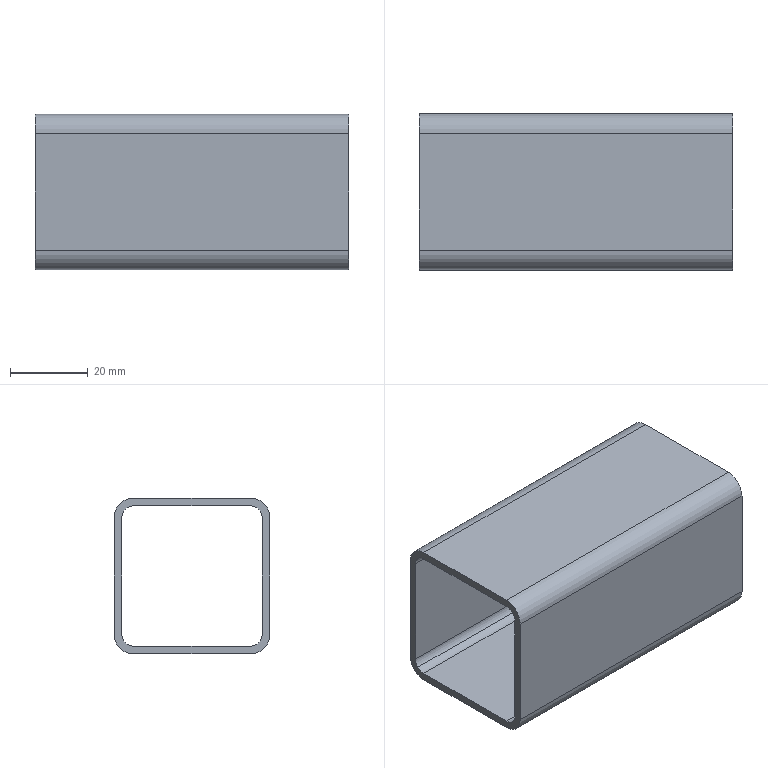Part | NX | features BREP 1 | 1 solid | 22 faces | box 80.5 x 40 x 40 mm | volume 23366 mm3 | cylinder 12 | plane 10 | commonest cylinder face diameters 6 x8 10 x4
STEP:
#1=CARTESIAN_POINT('',(2064.581,-321.621,69.879));
#2=VERTEX_POINT('',#1);
#3=CARTESIAN_POINT('',(2064.581,-319.5,69.));
#4=VERTEX_POINT('',#3);
#5=CARTESIAN_POINT('',(2064.581,-319.5,72.));
#6=DIRECTION('',(1.,0.,0.));
#7=DIRECTION('',(0.,0.,-1.));
#8=AXIS2_PLACEMENT_3D('',#5,#6,#7);
#9=CIRCLE('',#8,3.);
#10=EDGE_CURVE('',#2,#4,#9,.T.);
#11=ORIENTED_EDGE('',*,*,#10,.F.);
#12=CARTESIAN_POINT('',(2064.581,-322.5,72.));
#13=VERTEX_POINT('',#12);
#14=CARTESIAN_POINT('',(2064.581,-319.5,72.));
#15=DIRECTION('',(1.,0.,0.));
#16=DIRECTION('',(0.,0.,-1.));
#17=AXIS2_PLACEMENT_3D('',#14,#15,#16);
#18=CIRCLE('',#17,3.);
#19=EDGE_CURVE('',#13,#2,#18,.T.);
#20=ORIENTED_EDGE('',*,*,#19,.F.);
#21=CARTESIAN_POINT('',(2064.581,-322.5,102.));
#22=VERTEX_POINT('',#21);
#23=CARTESIAN_POINT('',(2064.581,-322.5,87.));
#24=DIRECTION('',(0.,0.,1.));
#25=VECTOR('',#24,1000.);
#26=LINE('',#23,#25);
#27=EDGE_CURVE('',#13,#22,#26,.T.);
#28=ORIENTED_EDGE('',*,*,#27,.T.);
#29=CARTESIAN_POINT('',(2064.581,-321.621,104.121));
#30=VERTEX_POINT('',#29);
#31=CARTESIAN_POINT('',(2064.581,-319.5,102.));
#32=DIRECTION('',(1.,0.,0.));
#33=DIRECTION('',(0.,0.,-1.));
#34=AXIS2_PLACEMENT_3D('',#31,#32,#33);
#35=CIRCLE('',#34,3.);
#36=EDGE_CURVE('',#30,#22,#35,.T.);
#37=ORIENTED_EDGE('',*,*,#36,.F.);
#38=CARTESIAN_POINT('',(2064.581,-319.5,105.));
#39=VERTEX_POINT('',#38);
#40=CARTESIAN_POINT('',(2064.581,-319.5,102.));
#41=DIRECTION('',(1.,0.,0.));
#42=DIRECTION('',(0.,0.,-1.));
#43=AXIS2_PLACEMENT_3D('',#40,#41,#42);
#44=CIRCLE('',#43,3.);
#45=EDGE_CURVE('',#39,#30,#44,.T.);
#46=ORIENTED_EDGE('',*,*,#45,.F.);
#47=CARTESIAN_POINT('',(2064.581,-289.5,105.));
#48=VERTEX_POINT('',#47);
#49=CARTESIAN_POINT('',(2064.581,-304.5,105.));
#50=DIRECTION('',(0.,-1.,0.));
#51=VECTOR('',#50,1000.);
#52=LINE('',#49,#51);
#53=EDGE_CURVE('',#48,#39,#52,.T.);
#54=ORIENTED_EDGE('',*,*,#53,.F.);
#55=CARTESIAN_POINT('',(2064.581,-287.378,104.121));
#56=VERTEX_POINT('',#55);
#57=CARTESIAN_POINT('',(2064.581,-289.5,102.));
#58=DIRECTION('',(1.,0.,0.));
#59=DIRECTION('',(0.,0.,-1.));
#60=AXIS2_PLACEMENT_3D('',#57,#58,#59);
#61=CIRCLE('',#60,3.);
#62=EDGE_CURVE('',#56,#48,#61,.T.);
#63=ORIENTED_EDGE('',*,*,#62,.F.);
#64=CARTESIAN_POINT('',(2064.581,-286.5,102.));
#65=VERTEX_POINT('',#64);
#66=CARTESIAN_POINT('',(2064.581,-289.5,102.));
#67=DIRECTION('',(1.,0.,0.));
#68=DIRECTION('',(0.,0.,-1.));
#69=AXIS2_PLACEMENT_3D('',#66,#67,#68);
#70=CIRCLE('',#69,3.);
#71=EDGE_CURVE('',#65,#56,#70,.T.);
#72=ORIENTED_EDGE('',*,*,#71,.F.);
#73=CARTESIAN_POINT('',(2064.581,-286.5,72.));
#74=VERTEX_POINT('',#73);
#75=CARTESIAN_POINT('',(2064.581,-286.5,87.));
#76=DIRECTION('',(0.,0.,-1.));
#77=VECTOR('',#76,1000.);
#78=LINE('',#75,#77);
#79=EDGE_CURVE('',#65,#74,#78,.T.);
#80=ORIENTED_EDGE('',*,*,#79,.T.);
#81=CARTESIAN_POINT('',(2064.581,-287.378,69.879));
#82=VERTEX_POINT('',#81);
#83=CARTESIAN_POINT('',(2064.581,-289.5,72.));
#84=DIRECTION('',(1.,0.,0.));
#85=DIRECTION('',(0.,0.,-1.));
#86=AXIS2_PLACEMENT_3D('',#83,#84,#85);
#87=CIRCLE('',#86,3.);
#88=EDGE_CURVE('',#82,#74,#87,.T.);
#89=ORIENTED_EDGE('',*,*,#88,.F.);
#90=CARTESIAN_POINT('',(2064.581,-289.5,69.));
#91=VERTEX_POINT('',#90);
#92=CARTESIAN_POINT('',(2064.581,-289.5,72.));
#93=DIRECTION('',(1.,0.,0.));
#94=DIRECTION('',(0.,0.,-1.));
#95=AXIS2_PLACEMENT_3D('',#92,#93,#94);
#96=CIRCLE('',#95,3.);
#97=EDGE_CURVE('',#91,#82,#96,.T.);
#98=ORIENTED_EDGE('',*,*,#97,.F.);
#99=CARTESIAN_POINT('',(2064.581,-304.5,69.));
#100=DIRECTION('',(0.,1.,0.));
#101=VECTOR('',#100,1000.);
#102=LINE('',#99,#101);
#103=EDGE_CURVE('',#4,#91,#102,.T.);
#104=ORIENTED_EDGE('',*,*,#103,.F.);
#105=EDGE_LOOP('',(#11,#20,#28,#37,#46,#54,#63,#72,#80,#89,#98,#104));
#106=FACE_BOUND('',#105,.T.);
#107=CARTESIAN_POINT('',(2064.581,-319.5,67.));
#108=VERTEX_POINT('',#107);
#109=CARTESIAN_POINT('',(2064.581,-289.5,67.));
#110=VERTEX_POINT('',#109);
#111=CARTESIAN_POINT('',(2064.581,-304.5,67.));
#112=DIRECTION('',(0.,1.,0.));
#113=VECTOR('',#112,1000.);
#114=LINE('',#111,#113);
#115=EDGE_CURVE('',#108,#110,#114,.T.);
#116=ORIENTED_EDGE('',*,*,#115,.T.);
#117=CARTESIAN_POINT('',(2064.581,-284.5,72.));
#118=VERTEX_POINT('',#117);
#119=CARTESIAN_POINT('',(2064.581,-289.5,72.));
#120=DIRECTION('',(1.,0.,0.));
#121=DIRECTION('',(0.,0.,-1.));
#122=AXIS2_PLACEMENT_3D('',#119,#120,#121);
#123=CIRCLE('',#122,5.);
#124=EDGE_CURVE('',#110,#118,#123,.T.);
#125=ORIENTED_EDGE('',*,*,#124,.T.);
#126=CARTESIAN_POINT('',(2064.581,-284.5,102.));
#127=VERTEX_POINT('',#126);
#128=CARTESIAN_POINT('',(2064.581,-284.5,87.));
#129=DIRECTION('',(0.,0.,-1.));
#130=VECTOR('',#129,1000.);
#131=LINE('',#128,#130);
#132=EDGE_CURVE('',#127,#118,#131,.T.);
#133=ORIENTED_EDGE('',*,*,#132,.F.);
#134=CARTESIAN_POINT('',(2064.581,-289.5,107.));
#135=VERTEX_POINT('',#134);
#136=CARTESIAN_POINT('',(2064.581,-289.5,102.));
#137=DIRECTION('',(1.,0.,0.));
#138=DIRECTION('',(0.,0.,-1.));
#139=AXIS2_PLACEMENT_3D('',#136,#137,#138);
#140=CIRCLE('',#139,5.);
#141=EDGE_CURVE('',#127,#135,#140,.T.);
#142=ORIENTED_EDGE('',*,*,#141,.T.);
#143=CARTESIAN_POINT('',(2064.581,-319.5,107.));
#144=VERTEX_POINT('',#143);
#145=CARTESIAN_POINT('',(2064.581,-304.5,107.));
#146=DIRECTION('',(0.,-1.,0.));
#147=VECTOR('',#146,1000.);
#148=LINE('',#145,#147);
#149=EDGE_CURVE('',#135,#144,#148,.T.);
#150=ORIENTED_EDGE('',*,*,#149,.T.);
#151=CARTESIAN_POINT('',(2064.581,-324.5,102.));
#152=VERTEX_POINT('',#151);
#153=CARTESIAN_POINT('',(2064.581,-319.5,102.));
#154=DIRECTION('',(1.,0.,0.));
#155=DIRECTION('',(0.,0.,-1.));
#156=AXIS2_PLACEMENT_3D('',#153,#154,#155);
#157=CIRCLE('',#156,5.);
#158=EDGE_CURVE('',#144,#152,#157,.T.);
#159=ORIENTED_EDGE('',*,*,#158,.T.);
#160=CARTESIAN_POINT('',(2064.581,-324.5,72.));
#161=VERTEX_POINT('',#160);
#162=CARTESIAN_POINT('',(2064.581,-324.5,87.));
#163=DIRECTION('',(0.,0.,1.));
#164=VECTOR('',#163,1000.);
#165=LINE('',#162,#164);
#166=EDGE_CURVE('',#161,#152,#165,.T.);
#167=ORIENTED_EDGE('',*,*,#166,.F.);
#168=CARTESIAN_POINT('',(2064.581,-319.5,72.));
#169=DIRECTION('',(1.,0.,0.));
#170=DIRECTION('',(0.,0.,-1.));
#171=AXIS2_PLACEMENT_3D('',#168,#169,#170);
#172=CIRCLE('',#171,5.);
#173=EDGE_CURVE('',#161,#108,#172,.T.);
#174=ORIENTED_EDGE('',*,*,#173,.T.);
#175=EDGE_LOOP('',(#116,#125,#133,#142,#150,#159,#167,#174));
#176=FACE_BOUND('',#175,.T.);
#177=CARTESIAN_POINT('',(2064.581,-306.25,87.));
#178=DIRECTION('',(1.,0.,0.));
#179=DIRECTION('',(0.,0.,-1.));
#180=AXIS2_PLACEMENT_3D('',#177,#178,#179);
#181=PLANE('',#180);
#182=ADVANCED_FACE('',(#106,#176),#181,.T.);
#183=CARTESIAN_POINT('',(1984.081,-286.5,72.));
#184=VERTEX_POINT('',#183);
#185=CARTESIAN_POINT('',(993.946,-286.5,72.));
#186=DIRECTION('',(1.,0.,0.));
#187=VECTOR('',#186,1000.);
#188=LINE('',#185,#187);
#189=EDGE_CURVE('',#184,#74,#188,.T.);
#190=ORIENTED_EDGE('',*,*,#189,.T.);
#191=ORIENTED_EDGE('',*,*,#79,.F.);
#192=CARTESIAN_POINT('',(1984.081,-286.5,102.));
#193=VERTEX_POINT('',#192);
#194=CARTESIAN_POINT('',(993.946,-286.5,102.));
#195=DIRECTION('',(1.,0.,0.));
#196=VECTOR('',#195,1000.);
#197=LINE('',#194,#196);
#198=EDGE_CURVE('',#193,#65,#197,.T.);
#199=ORIENTED_EDGE('',*,*,#198,.F.);
#200=CARTESIAN_POINT('',(1984.081,-286.5,87.));
#201=DIRECTION('',(0.,0.,-1.));
#202=VECTOR('',#201,1000.);
#203=LINE('',#200,#202);
#204=EDGE_CURVE('',#193,#184,#203,.T.);
#205=ORIENTED_EDGE('',*,*,#204,.T.);
#206=EDGE_LOOP('',(#190,#191,#199,#205));
#207=FACE_BOUND('',#206,.T.);
#208=CARTESIAN_POINT('',(601.965,-286.5,127.));
#209=DIRECTION('',(0.,-1.,0.));
#210=DIRECTION('',(0.,0.,-1.));
#211=AXIS2_PLACEMENT_3D('',#208,#209,#210);
#212=PLANE('',#211);
#213=ADVANCED_FACE('',(#207),#212,.T.);
#214=ORIENTED_EDGE('',*,*,#88,.T.);
#215=ORIENTED_EDGE('',*,*,#189,.F.);
#216=CARTESIAN_POINT('',(1984.081,-287.378,69.879));
#217=VERTEX_POINT('',#216);
#218=CARTESIAN_POINT('',(1984.081,-289.5,72.));
#219=DIRECTION('',(1.,0.,0.));
#220=DIRECTION('',(0.,0.,-1.));
#221=AXIS2_PLACEMENT_3D('',#218,#219,#220);
#222=CIRCLE('',#221,3.);
#223=EDGE_CURVE('',#217,#184,#222,.T.);
#224=ORIENTED_EDGE('',*,*,#223,.F.);
#225=CARTESIAN_POINT('',(993.946,-287.378,69.879));
#226=DIRECTION('',(1.,0.,0.));
#227=VECTOR('',#226,1000.);
#228=LINE('',#225,#227);
#229=EDGE_CURVE('',#217,#82,#228,.T.);
#230=ORIENTED_EDGE('',*,*,#229,.T.);
#231=EDGE_LOOP('',(#214,#215,#224,#230));
#232=FACE_BOUND('',#231,.T.);
#233=CARTESIAN_POINT('',(993.946,-289.5,72.));
#234=DIRECTION('',(1.,0.,0.));
#235=DIRECTION('',(0.,0.7071,-0.7071));
#236=AXIS2_PLACEMENT_3D('',#233,#234,#235);
#237=CYLINDRICAL_SURFACE('',#236,3.);
#238=ADVANCED_FACE('',(#232),#237,.F.);
#239=CARTESIAN_POINT('',(1984.081,-289.5,69.));
#240=VERTEX_POINT('',#239);
#241=CARTESIAN_POINT('',(1984.081,-289.5,72.));
#242=DIRECTION('',(1.,0.,0.));
#243=DIRECTION('',(0.,0.,-1.));
#244=AXIS2_PLACEMENT_3D('',#241,#242,#243);
#245=CIRCLE('',#244,3.);
#246=EDGE_CURVE('',#240,#217,#245,.T.);
#247=ORIENTED_EDGE('',*,*,#246,.F.);
#248=CARTESIAN_POINT('',(2024.331,-289.5,69.));
#249=DIRECTION('',(1.,0.,0.));
#250=VECTOR('',#249,1000.);
#251=LINE('',#248,#250);
#252=EDGE_CURVE('',#240,#91,#251,.T.);
#253=ORIENTED_EDGE('',*,*,#252,.T.);
#254=ORIENTED_EDGE('',*,*,#97,.T.);
#255=ORIENTED_EDGE('',*,*,#229,.F.);
#256=EDGE_LOOP('',(#247,#253,#254,#255));
#257=FACE_BOUND('',#256,.T.);
#258=CARTESIAN_POINT('',(993.946,-289.5,72.));
#259=DIRECTION('',(1.,0.,0.));
#260=DIRECTION('',(0.,-0.7071,0.7071));
#261=AXIS2_PLACEMENT_3D('',#258,#259,#260);
#262=CYLINDRICAL_SURFACE('',#261,3.);
#263=ADVANCED_FACE('',(#257),#262,.F.);
#264=CARTESIAN_POINT('',(1984.081,-319.5,69.));
#265=VERTEX_POINT('',#264);
#266=CARTESIAN_POINT('',(1984.081,-304.5,69.));
#267=DIRECTION('',(0.,1.,0.));
#268=VECTOR('',#267,1000.);
#269=LINE('',#266,#268);
#270=EDGE_CURVE('',#265,#240,#269,.T.);
#271=ORIENTED_EDGE('',*,*,#270,.F.);
#272=CARTESIAN_POINT('',(993.946,-319.5,69.));
#273=DIRECTION('',(1.,0.,0.));
#274=VECTOR('',#273,1000.);
#275=LINE('',#272,#274);
#276=EDGE_CURVE('',#265,#4,#275,.T.);
#277=ORIENTED_EDGE('',*,*,#276,.T.);
#278=ORIENTED_EDGE('',*,*,#103,.T.);
#279=ORIENTED_EDGE('',*,*,#252,.F.);
#280=EDGE_LOOP('',(#271,#277,#278,#279));
#281=FACE_BOUND('',#280,.T.);
#282=CARTESIAN_POINT('',(601.965,-344.5,69.));
#283=DIRECTION('',(0.,0.,-1.));
#284=DIRECTION('',(0.,1.,0.));
#285=AXIS2_PLACEMENT_3D('',#282,#283,#284);
#286=PLANE('',#285);
#287=ADVANCED_FACE('',(#281),#286,.F.);
#288=ORIENTED_EDGE('',*,*,#10,.T.);
#289=ORIENTED_EDGE('',*,*,#276,.F.);
#290=CARTESIAN_POINT('',(1984.081,-321.621,69.879));
#291=VERTEX_POINT('',#290);
#292=CARTESIAN_POINT('',(1984.081,-319.5,72.));
#293=DIRECTION('',(1.,0.,0.));
#294=DIRECTION('',(0.,0.,-1.));
#295=AXIS2_PLACEMENT_3D('',#292,#293,#294);
#296=CIRCLE('',#295,3.);
#297=EDGE_CURVE('',#291,#265,#296,.T.);
#298=ORIENTED_EDGE('',*,*,#297,.F.);
#299=CARTESIAN_POINT('',(993.946,-321.621,69.879));
#300=DIRECTION('',(1.,0.,0.));
#301=VECTOR('',#300,1000.);
#302=LINE('',#299,#301);
#303=EDGE_CURVE('',#291,#2,#302,.T.);
#304=ORIENTED_EDGE('',*,*,#303,.T.);
#305=EDGE_LOOP('',(#288,#289,#298,#304));
#306=FACE_BOUND('',#305,.T.);
#307=CARTESIAN_POINT('',(993.946,-319.5,72.));
#308=DIRECTION('',(1.,0.,0.));
#309=DIRECTION('',(0.,-0.7071,-0.7071));
#310=AXIS2_PLACEMENT_3D('',#307,#308,#309);
#311=CYLINDRICAL_SURFACE('',#310,3.);
#312=ADVANCED_FACE('',(#306),#311,.F.);
#313=CARTESIAN_POINT('',(1984.081,-322.5,72.));
#314=VERTEX_POINT('',#313);
#315=CARTESIAN_POINT('',(1984.081,-319.5,72.));
#316=DIRECTION('',(1.,0.,0.));
#317=DIRECTION('',(0.,0.,-1.));
#318=AXIS2_PLACEMENT_3D('',#315,#316,#317);
#319=CIRCLE('',#318,3.);
#320=EDGE_CURVE('',#314,#291,#319,.T.);
#321=ORIENTED_EDGE('',*,*,#320,.F.);
#322=CARTESIAN_POINT('',(2024.331,-322.5,72.));
#323=DIRECTION('',(1.,0.,0.));
#324=VECTOR('',#323,1000.);
#325=LINE('',#322,#324);
#326=EDGE_CURVE('',#314,#13,#325,.T.);
#327=ORIENTED_EDGE('',*,*,#326,.T.);
#328=ORIENTED_EDGE('',*,*,#19,.T.);
#329=ORIENTED_EDGE('',*,*,#303,.F.);
#330=EDGE_LOOP('',(#321,#327,#328,#329));
#331=FACE_BOUND('',#330,.T.);
#332=CARTESIAN_POINT('',(993.946,-319.5,72.));
#333=DIRECTION('',(1.,0.,0.));
#334=DIRECTION('',(0.,0.7071,0.7071));
#335=AXIS2_PLACEMENT_3D('',#332,#333,#334);
#336=CYLINDRICAL_SURFACE('',#335,3.);
#337=ADVANCED_FACE('',(#331),#336,.F.);
#338=CARTESIAN_POINT('',(1984.081,-322.5,102.));
#339=VERTEX_POINT('',#338);
#340=CARTESIAN_POINT('',(993.946,-322.5,102.));
#341=DIRECTION('',(1.,0.,0.));
#342=VECTOR('',#341,1000.);
#343=LINE('',#340,#342);
#344=EDGE_CURVE('',#339,#22,#343,.T.);
#345=ORIENTED_EDGE('',*,*,#344,.T.);
#346=ORIENTED_EDGE('',*,*,#27,.F.);
#347=ORIENTED_EDGE('',*,*,#326,.F.);
#348=CARTESIAN_POINT('',(1984.081,-322.5,87.));
#349=DIRECTION('',(0.,0.,1.));
#350=VECTOR('',#349,1000.);
#351=LINE('',#348,#350);
#352=EDGE_CURVE('',#314,#339,#351,.T.);
#353=ORIENTED_EDGE('',*,*,#352,.T.);
#354=EDGE_LOOP('',(#345,#346,#347,#353));
#355=FACE_BOUND('',#354,.T.);
#356=CARTESIAN_POINT('',(601.965,-322.5,47.));
#357=DIRECTION('',(0.,1.,0.));
#358=DIRECTION('',(0.,0.,1.));
#359=AXIS2_PLACEMENT_3D('',#356,#357,#358);
#360=PLANE('',#359);
#361=ADVANCED_FACE('',(#355),#360,.T.);
#362=ORIENTED_EDGE('',*,*,#36,.T.);
#363=ORIENTED_EDGE('',*,*,#344,.F.);
#364=CARTESIAN_POINT('',(1984.081,-321.621,104.121));
#365=VERTEX_POINT('',#364);
#366=CARTESIAN_POINT('',(1984.081,-319.5,102.));
#367=DIRECTION('',(1.,0.,0.));
#368=DIRECTION('',(0.,0.,-1.));
#369=AXIS2_PLACEMENT_3D('',#366,#367,#368);
#370=CIRCLE('',#369,3.);
#371=EDGE_CURVE('',#365,#339,#370,.T.);
#372=ORIENTED_EDGE('',*,*,#371,.F.);
#373=CARTESIAN_POINT('',(993.946,-321.621,104.121));
#374=DIRECTION('',(1.,0.,0.));
#375=VECTOR('',#374,1000.);
#376=LINE('',#373,#375);
#377=EDGE_CURVE('',#365,#30,#376,.T.);
#378=ORIENTED_EDGE('',*,*,#377,.T.);
#379=EDGE_LOOP('',(#362,#363,#372,#378));
#380=FACE_BOUND('',#379,.T.);
#381=CARTESIAN_POINT('',(993.946,-319.5,102.));
#382=DIRECTION('',(1.,0.,0.));
#383=DIRECTION('',(0.,-0.7071,0.7071));
#384=AXIS2_PLACEMENT_3D('',#381,#382,#383);
#385=CYLINDRICAL_SURFACE('',#384,3.);
#386=ADVANCED_FACE('',(#380),#385,.F.);
#387=CARTESIAN_POINT('',(1984.081,-319.5,105.));
#388=VERTEX_POINT('',#387);
#389=CARTESIAN_POINT('',(1984.081,-319.5,102.));
#390=DIRECTION('',(1.,0.,0.));
#391=DIRECTION('',(0.,0.,-1.));
#392=AXIS2_PLACEMENT_3D('',#389,#390,#391);
#393=CIRCLE('',#392,3.);
#394=EDGE_CURVE('',#388,#365,#393,.T.);
#395=ORIENTED_EDGE('',*,*,#394,.F.);
#396=CARTESIAN_POINT('',(2024.331,-319.5,105.));
#397=DIRECTION('',(1.,0.,0.));
#398=VECTOR('',#397,1000.);
#399=LINE('',#396,#398);
#400=EDGE_CURVE('',#388,#39,#399,.T.);
#401=ORIENTED_EDGE('',*,*,#400,.T.);
#402=ORIENTED_EDGE('',*,*,#45,.T.);
#403=ORIENTED_EDGE('',*,*,#377,.F.);
#404=EDGE_LOOP('',(#395,#401,#402,#403));
#405=FACE_BOUND('',#404,.T.);
#406=CARTESIAN_POINT('',(993.946,-319.5,102.));
#407=DIRECTION('',(1.,0.,0.));
#408=DIRECTION('',(0.,0.7071,-0.7071));
#409=AXIS2_PLACEMENT_3D('',#406,#407,#408);
#410=CYLINDRICAL_SURFACE('',#409,3.);
#411=ADVANCED_FACE('',(#405),#410,.F.);
#412=CARTESIAN_POINT('',(1984.081,-289.5,105.));
#413=VERTEX_POINT('',#412);
#414=CARTESIAN_POINT('',(1984.081,-304.5,105.));
#415=DIRECTION('',(0.,-1.,0.));
#416=VECTOR('',#415,1000.);
#417=LINE('',#414,#416);
#418=EDGE_CURVE('',#413,#388,#417,.T.);
#419=ORIENTED_EDGE('',*,*,#418,.F.);
#420=CARTESIAN_POINT('',(993.946,-289.5,105.));
#421=DIRECTION('',(1.,0.,0.));
#422=VECTOR('',#421,1000.);
#423=LINE('',#420,#422);
#424=EDGE_CURVE('',#413,#48,#423,.T.);
#425=ORIENTED_EDGE('',*,*,#424,.T.);
#426=ORIENTED_EDGE('',*,*,#53,.T.);
#427=ORIENTED_EDGE('',*,*,#400,.F.);
#428=EDGE_LOOP('',(#419,#425,#426,#427));
#429=FACE_BOUND('',#428,.T.);
#430=CARTESIAN_POINT('',(601.965,-264.5,105.));
#431=DIRECTION('',(0.,0.,1.));
#432=DIRECTION('',(0.,-1.,0.));
#433=AXIS2_PLACEMENT_3D('',#430,#431,#432);
#434=PLANE('',#433);
#435=ADVANCED_FACE('',(#429),#434,.F.);
#436=ORIENTED_EDGE('',*,*,#62,.T.);
#437=ORIENTED_EDGE('',*,*,#424,.F.);
#438=CARTESIAN_POINT('',(1984.081,-287.378,104.121));
#439=VERTEX_POINT('',#438);
#440=CARTESIAN_POINT('',(1984.081,-289.5,102.));
#441=DIRECTION('',(1.,0.,0.));
#442=DIRECTION('',(0.,0.,-1.));
#443=AXIS2_PLACEMENT_3D('',#440,#441,#442);
#444=CIRCLE('',#443,3.);
#445=EDGE_CURVE('',#439,#413,#444,.T.);
#446=ORIENTED_EDGE('',*,*,#445,.F.);
#447=CARTESIAN_POINT('',(993.946,-287.378,104.121));
#448=DIRECTION('',(1.,0.,0.));
#449=VECTOR('',#448,1000.);
#450=LINE('',#447,#449);
#451=EDGE_CURVE('',#439,#56,#450,.T.);
#452=ORIENTED_EDGE('',*,*,#451,.T.);
#453=EDGE_LOOP('',(#436,#437,#446,#452));
#454=FACE_BOUND('',#453,.T.);
#455=CARTESIAN_POINT('',(993.946,-289.5,102.));
#456=DIRECTION('',(1.,0.,0.));
#457=DIRECTION('',(0.,0.7071,0.7071));
#458=AXIS2_PLACEMENT_3D('',#455,#456,#457);
#459=CYLINDRICAL_SURFACE('',#458,3.);
#460=ADVANCED_FACE('',(#454),#459,.F.);
#461=CARTESIAN_POINT('',(1984.081,-289.5,102.));
#462=DIRECTION('',(1.,0.,0.));
#463=DIRECTION('',(0.,0.,-1.));
#464=AXIS2_PLACEMENT_3D('',#461,#462,#463);
#465=CIRCLE('',#464,3.);
#466=EDGE_CURVE('',#193,#439,#465,.T.);
#467=ORIENTED_EDGE('',*,*,#466,.F.);
#468=ORIENTED_EDGE('',*,*,#198,.T.);
#469=ORIENTED_EDGE('',*,*,#71,.T.);
#470=ORIENTED_EDGE('',*,*,#451,.F.);
#471=EDGE_LOOP('',(#467,#468,#469,#470));
#472=FACE_BOUND('',#471,.T.);
#473=CARTESIAN_POINT('',(993.946,-289.5,102.));
#474=DIRECTION('',(1.,0.,0.));
#475=DIRECTION('',(0.,-0.7071,-0.7071));
#476=AXIS2_PLACEMENT_3D('',#473,#474,#475);
#477=CYLINDRICAL_SURFACE('',#476,3.);
#478=ADVANCED_FACE('',(#472),#477,.F.);
#479=CARTESIAN_POINT('',(1984.081,-289.5,107.));
#480=VERTEX_POINT('',#479);
#481=CARTESIAN_POINT('',(2024.331,-289.5,107.));
#482=DIRECTION('',(1.,0.,0.));
#483=VECTOR('',#482,1000.);
#484=LINE('',#481,#483);
#485=EDGE_CURVE('',#480,#135,#484,.T.);
#486=ORIENTED_EDGE('',*,*,#485,.T.);
#487=ORIENTED_EDGE('',*,*,#141,.F.);
#488=CARTESIAN_POINT('',(1984.081,-284.5,102.));
#489=VERTEX_POINT('',#488);
#490=CARTESIAN_POINT('',(2024.331,-284.5,102.));
#491=DIRECTION('',(1.,0.,0.));
#492=VECTOR('',#491,1000.);
#493=LINE('',#490,#492);
#494=EDGE_CURVE('',#489,#127,#493,.T.);
#495=ORIENTED_EDGE('',*,*,#494,.F.);
#496=CARTESIAN_POINT('',(1984.081,-289.5,102.));
#497=DIRECTION('',(1.,0.,0.));
#498=DIRECTION('',(0.,0.,-1.));
#499=AXIS2_PLACEMENT_3D('',#496,#497,#498);
#500=CIRCLE('',#499,5.);
#501=EDGE_CURVE('',#489,#480,#500,.T.);
#502=ORIENTED_EDGE('',*,*,#501,.T.);
#503=EDGE_LOOP('',(#486,#487,#495,#502));
#504=FACE_BOUND('',#503,.T.);
#505=CARTESIAN_POINT('',(993.946,-289.5,102.));
#506=DIRECTION('',(1.,0.,0.));
#507=DIRECTION('',(0.,1.,0.));
#508=AXIS2_PLACEMENT_3D('',#505,#506,#507);
#509=CYLINDRICAL_SURFACE('',#508,5.);
#510=ADVANCED_FACE('',(#504),#509,.T.);
#511=CARTESIAN_POINT('',(1984.081,-319.5,107.));
#512=VERTEX_POINT('',#511);
#513=CARTESIAN_POINT('',(993.946,-319.5,107.));
#514=DIRECTION('',(1.,0.,0.));
#515=VECTOR('',#514,1000.);
#516=LINE('',#513,#515);
#517=EDGE_CURVE('',#512,#144,#516,.T.);
#518=ORIENTED_EDGE('',*,*,#517,.T.);
#519=ORIENTED_EDGE('',*,*,#149,.F.);
#520=ORIENTED_EDGE('',*,*,#485,.F.);
#521=CARTESIAN_POINT('',(1984.081,-304.5,107.));
#522=DIRECTION('',(0.,-1.,0.));
#523=VECTOR('',#522,1000.);
#524=LINE('',#521,#523);
#525=EDGE_CURVE('',#480,#512,#524,.T.);
#526=ORIENTED_EDGE('',*,*,#525,.T.);
#527=EDGE_LOOP('',(#518,#519,#520,#526));
#528=FACE_BOUND('',#527,.T.);
#529=CARTESIAN_POINT('',(601.965,-264.5,107.));
#530=DIRECTION('',(0.,0.,1.));
#531=DIRECTION('',(0.,-1.,0.));
#532=AXIS2_PLACEMENT_3D('',#529,#530,#531);
#533=PLANE('',#532);
#534=ADVANCED_FACE('',(#528),#533,.T.);
#535=CARTESIAN_POINT('',(1984.081,-324.5,102.));
#536=VERTEX_POINT('',#535);
#537=CARTESIAN_POINT('',(2024.331,-324.5,102.));
#538=DIRECTION('',(1.,0.,0.));
#539=VECTOR('',#538,1000.);
#540=LINE('',#537,#539);
#541=EDGE_CURVE('',#536,#152,#540,.T.);
#542=ORIENTED_EDGE('',*,*,#541,.T.);
#543=ORIENTED_EDGE('',*,*,#158,.F.);
#544=ORIENTED_EDGE('',*,*,#517,.F.);
#545=CARTESIAN_POINT('',(1984.081,-319.5,102.));
#546=DIRECTION('',(1.,0.,0.));
#547=DIRECTION('',(0.,0.,-1.));
#548=AXIS2_PLACEMENT_3D('',#545,#546,#547);
#549=CIRCLE('',#548,5.);
#550=EDGE_CURVE('',#512,#536,#549,.T.);
#551=ORIENTED_EDGE('',*,*,#550,.T.);
#552=EDGE_LOOP('',(#542,#543,#544,#551));
#553=FACE_BOUND('',#552,.T.);
#554=CARTESIAN_POINT('',(993.946,-319.5,102.));
#555=DIRECTION('',(1.,0.,0.));
#556=DIRECTION('',(0.,0.,1.));
#557=AXIS2_PLACEMENT_3D('',#554,#555,#556);
#558=CYLINDRICAL_SURFACE('',#557,5.);
#559=ADVANCED_FACE('',(#553),#558,.T.);
#560=CARTESIAN_POINT('',(1984.081,-324.5,72.));
#561=VERTEX_POINT('',#560);
#562=CARTESIAN_POINT('',(1984.081,-324.5,87.));
#563=DIRECTION('',(0.,0.,1.));
#564=VECTOR('',#563,1000.);
#565=LINE('',#562,#564);
#566=EDGE_CURVE('',#561,#536,#565,.T.);
#567=ORIENTED_EDGE('',*,*,#566,.F.);
#568=CARTESIAN_POINT('',(993.946,-324.5,72.));
#569=DIRECTION('',(1.,0.,0.));
#570=VECTOR('',#569,1000.);
#571=LINE('',#568,#570);
#572=EDGE_CURVE('',#561,#161,#571,.T.);
#573=ORIENTED_EDGE('',*,*,#572,.T.);
#574=ORIENTED_EDGE('',*,*,#166,.T.);
#575=ORIENTED_EDGE('',*,*,#541,.F.);
#576=EDGE_LOOP('',(#567,#573,#574,#575));
#577=FACE_BOUND('',#576,.T.);
#578=CARTESIAN_POINT('',(601.965,-324.5,47.));
#579=DIRECTION('',(0.,1.,0.));
#580=DIRECTION('',(0.,0.,1.));
#581=AXIS2_PLACEMENT_3D('',#578,#579,#580);
#582=PLANE('',#581);
#583=ADVANCED_FACE('',(#577),#582,.F.);
#584=CARTESIAN_POINT('',(1984.081,-319.5,67.));
#585=VERTEX_POINT('',#584);
#586=CARTESIAN_POINT('',(2024.331,-319.5,67.));
#587=DIRECTION('',(1.,0.,0.));
#588=VECTOR('',#587,1000.);
#589=LINE('',#586,#588);
#590=EDGE_CURVE('',#585,#108,#589,.T.);
#591=ORIENTED_EDGE('',*,*,#590,.T.);
#592=ORIENTED_EDGE('',*,*,#173,.F.);
#593=ORIENTED_EDGE('',*,*,#572,.F.);
#594=CARTESIAN_POINT('',(1984.081,-319.5,72.));
#595=DIRECTION('',(1.,0.,0.));
#596=DIRECTION('',(0.,0.,-1.));
#597=AXIS2_PLACEMENT_3D('',#594,#595,#596);
#598=CIRCLE('',#597,5.);
#599=EDGE_CURVE('',#561,#585,#598,.T.);
#600=ORIENTED_EDGE('',*,*,#599,.T.);
#601=EDGE_LOOP('',(#591,#592,#593,#600));
#602=FACE_BOUND('',#601,.T.);
#603=CARTESIAN_POINT('',(993.946,-319.5,72.));
#604=DIRECTION('',(1.,0.,0.));
#605=DIRECTION('',(0.,-1.,0.));
#606=AXIS2_PLACEMENT_3D('',#603,#604,#605);
#607=CYLINDRICAL_SURFACE('',#606,5.);
#608=ADVANCED_FACE('',(#602),#607,.T.);
#609=CARTESIAN_POINT('',(1984.081,-289.5,67.));
#610=VERTEX_POINT('',#609);
#611=CARTESIAN_POINT('',(993.946,-289.5,67.));
#612=DIRECTION('',(1.,0.,0.));
#613=VECTOR('',#612,1000.);
#614=LINE('',#611,#613);
#615=EDGE_CURVE('',#610,#110,#614,.T.);
#616=ORIENTED_EDGE('',*,*,#615,.T.);
#617=ORIENTED_EDGE('',*,*,#115,.F.);
#618=ORIENTED_EDGE('',*,*,#590,.F.);
#619=CARTESIAN_POINT('',(1984.081,-304.5,67.));
#620=DIRECTION('',(0.,1.,0.));
#621=VECTOR('',#620,1000.);
#622=LINE('',#619,#621);
#623=EDGE_CURVE('',#585,#610,#622,.T.);
#624=ORIENTED_EDGE('',*,*,#623,.T.);
#625=EDGE_LOOP('',(#616,#617,#618,#624));
#626=FACE_BOUND('',#625,.T.);
#627=CARTESIAN_POINT('',(601.965,-344.5,67.));
#628=DIRECTION('',(0.,0.,-1.));
#629=DIRECTION('',(0.,1.,0.));
#630=AXIS2_PLACEMENT_3D('',#627,#628,#629);
#631=PLANE('',#630);
#632=ADVANCED_FACE('',(#626),#631,.T.);
#633=CARTESIAN_POINT('',(1984.081,-284.5,72.));
#634=VERTEX_POINT('',#633);
#635=CARTESIAN_POINT('',(2024.331,-284.5,72.));
#636=DIRECTION('',(1.,0.,0.));
#637=VECTOR('',#636,1000.);
#638=LINE('',#635,#637);
#639=EDGE_CURVE('',#634,#118,#638,.T.);
#640=ORIENTED_EDGE('',*,*,#639,.T.);
#641=ORIENTED_EDGE('',*,*,#124,.F.);
#642=ORIENTED_EDGE('',*,*,#615,.F.);
#643=CARTESIAN_POINT('',(1984.081,-289.5,72.));
#644=DIRECTION('',(1.,0.,0.));
#645=DIRECTION('',(0.,0.,-1.));
#646=AXIS2_PLACEMENT_3D('',#643,#644,#645);
#647=CIRCLE('',#646,5.);
#648=EDGE_CURVE('',#610,#634,#647,.T.);
#649=ORIENTED_EDGE('',*,*,#648,.T.);
#650=EDGE_LOOP('',(#640,#641,#642,#649));
#651=FACE_BOUND('',#650,.T.);
#652=CARTESIAN_POINT('',(993.946,-289.5,72.));
#653=DIRECTION('',(1.,0.,0.));
#654=DIRECTION('',(0.,0.,-1.));
#655=AXIS2_PLACEMENT_3D('',#652,#653,#654);
#656=CYLINDRICAL_SURFACE('',#655,5.);
#657=ADVANCED_FACE('',(#651),#656,.T.);
#658=CARTESIAN_POINT('',(1984.081,-284.5,87.));
#659=DIRECTION('',(0.,0.,-1.));
#660=VECTOR('',#659,1000.);
#661=LINE('',#658,#660);
#662=EDGE_CURVE('',#489,#634,#661,.T.);
#663=ORIENTED_EDGE('',*,*,#662,.F.);
#664=ORIENTED_EDGE('',*,*,#494,.T.);
#665=ORIENTED_EDGE('',*,*,#132,.T.);
#666=ORIENTED_EDGE('',*,*,#639,.F.);
#667=EDGE_LOOP('',(#663,#664,#665,#666));
#668=FACE_BOUND('',#667,.T.);
#669=CARTESIAN_POINT('',(601.965,-284.5,127.));
#670=DIRECTION('',(0.,-1.,0.));
#671=DIRECTION('',(0.,0.,-1.));
#672=AXIS2_PLACEMENT_3D('',#669,#670,#671);
#673=PLANE('',#672);
#674=ADVANCED_FACE('',(#668),#673,.F.);
#675=ORIENTED_EDGE('',*,*,#466,.T.);
#676=ORIENTED_EDGE('',*,*,#445,.T.);
#677=ORIENTED_EDGE('',*,*,#418,.T.);
#678=ORIENTED_EDGE('',*,*,#394,.T.);
#679=ORIENTED_EDGE('',*,*,#371,.T.);
#680=ORIENTED_EDGE('',*,*,#352,.F.);
#681=ORIENTED_EDGE('',*,*,#320,.T.);
#682=ORIENTED_EDGE('',*,*,#297,.T.);
#683=ORIENTED_EDGE('',*,*,#270,.T.);
#684=ORIENTED_EDGE('',*,*,#246,.T.);
#685=ORIENTED_EDGE('',*,*,#223,.T.);
#686=ORIENTED_EDGE('',*,*,#204,.F.);
#687=EDGE_LOOP('',(#675,#676,#677,#678,#679,#680,#681,#682,#683,#684,#685,#686));
#688=FACE_BOUND('',#687,.T.);
#689=ORIENTED_EDGE('',*,*,#662,.T.);
#690=ORIENTED_EDGE('',*,*,#648,.F.);
#691=ORIENTED_EDGE('',*,*,#623,.F.);
#692=ORIENTED_EDGE('',*,*,#599,.F.);
#693=ORIENTED_EDGE('',*,*,#566,.T.);
#694=ORIENTED_EDGE('',*,*,#550,.F.);
#695=ORIENTED_EDGE('',*,*,#525,.F.);
#696=ORIENTED_EDGE('',*,*,#501,.F.);
#697=EDGE_LOOP('',(#689,#690,#691,#692,#693,#694,#695,#696));
#698=FACE_BOUND('',#697,.T.);
#699=CARTESIAN_POINT('',(1984.081,-306.25,45.));
#700=DIRECTION('',(1.,0.,0.));
#701=DIRECTION('',(0.,0.,-1.));
#702=AXIS2_PLACEMENT_3D('',#699,#700,#701);
#703=PLANE('',#702);
#704=ADVANCED_FACE('',(#688,#698),#703,.F.);
#705=CLOSED_SHELL('',(#182,#213,#238,#263,#287,#312,#337,#361,#386,#411,#435,#460,#478,#510,#534,#559,#583,#608,#632,#657,#674,#704));
#706=MANIFOLD_SOLID_BREP('',#705);
#707=(LENGTH_UNIT()NAMED_UNIT(*)SI_UNIT(.MILLI.,.METRE.));
#708=UNCERTAINTY_MEASURE_WITH_UNIT(LENGTH_MEASURE(0.00001),#707,'','');
#709=(NAMED_UNIT(*)PLANE_ANGLE_UNIT()SI_UNIT($,.RADIAN.));
#710=(NAMED_UNIT(*)SI_UNIT($,.STERADIAN.)SOLID_ANGLE_UNIT());
#711=(GEOMETRIC_REPRESENTATION_CONTEXT(3)GLOBAL_UNCERTAINTY_ASSIGNED_CONTEXT((#708))GLOBAL_UNIT_ASSIGNED_CONTEXT((#707,#709,#710))REPRESENTATION_CONTEXT('',''));
#712=ADVANCED_BREP_SHAPE_REPRESENTATION('',(#706),#711);